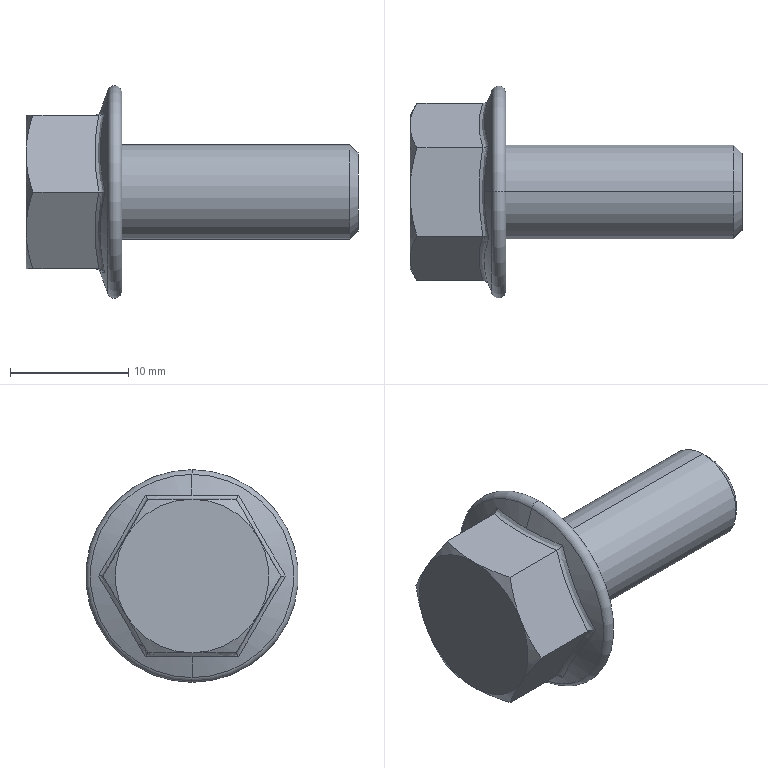Part | STEP file | heavy hex flange screw_am_B18.2.3.9M - Heavy hex flange screw, M8 x 1.25 x 20 --20N | 1 solid | 29 faces | box 28.1 x 18 x 18 mm | volume 2330 mm3 | cone 10 | plane 9 | spline 6 | torus 2 | cylinder 2 | commonest cylinder face diameters 8 x2